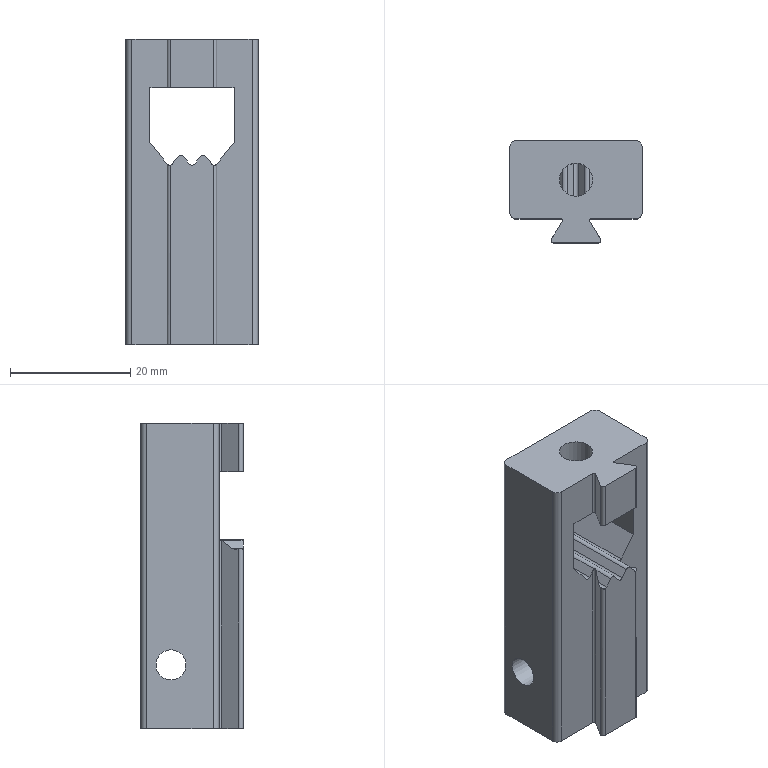Part | STEP file | 200 mesh_id1934 | 1 solid | 45 faces | box 22 x 17 x 50.8 mm | volume 12732 mm3 | plane 24 | cylinder 21 | commonest cylinder face diameters 1.04 x5 0.6 x4 1 x4 2 x4 1.2 x2 5.01 x1